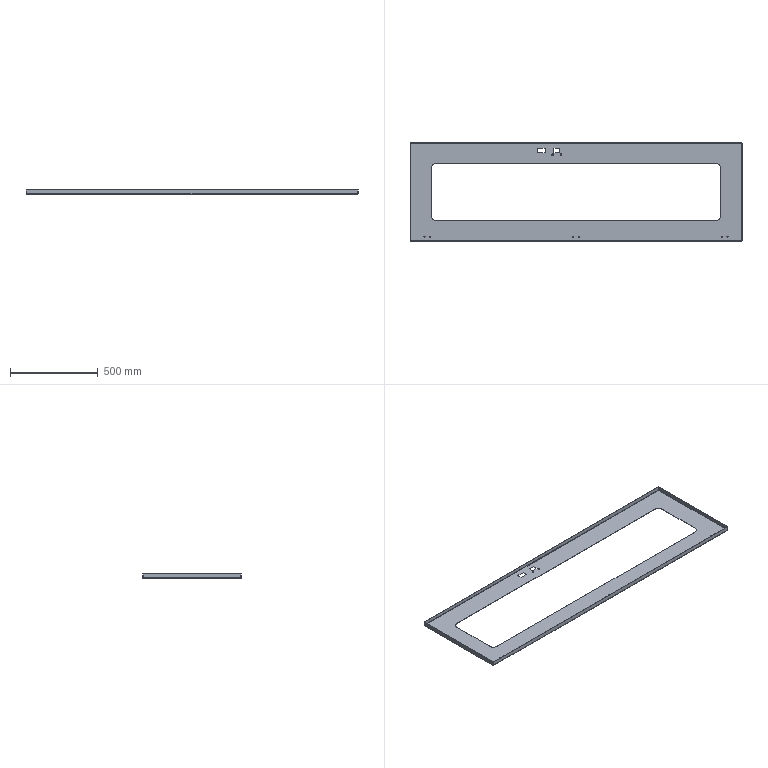Part | SolidWorks | features ICE 3, Extrusion 1, FlatPattern 1, FlattenBends 1, ProcessBends 1, Rip 1, SheetMetal 1, Shell 1 | 1 solid | 94 faces | box 1891 x 561 x 25 mm | volume 1274365 mm3 | plane 66 | cylinder 28 | commonest cylinder face diameters 6 x16 2 x4 10 x4 50 x4